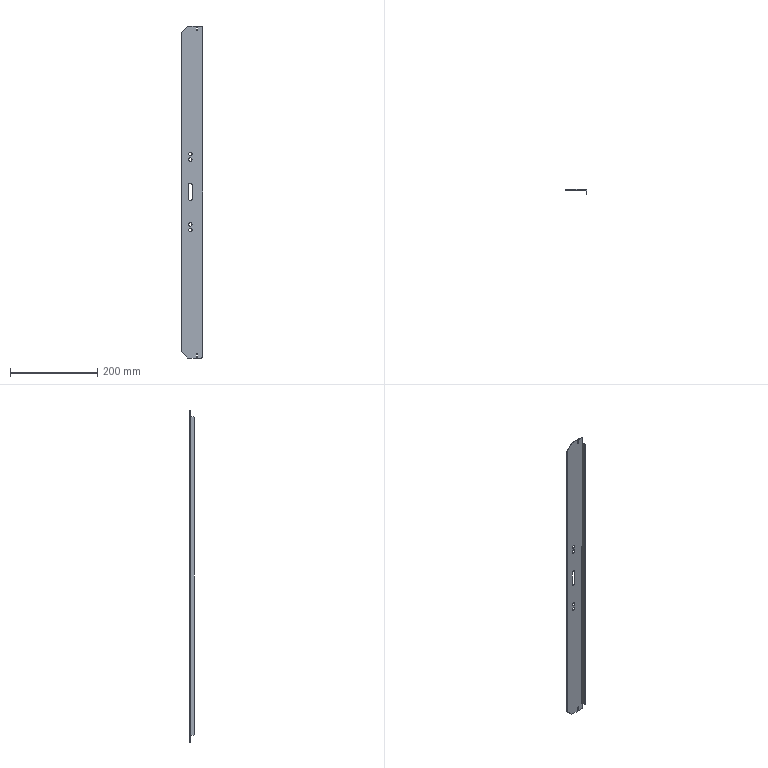Part | SolidWorks | features BaseBody 1 | 1 solid | 39 faces | box 49.5 x 10.7 x 760 mm | volume 52509 mm3 | cylinder 21 | plane 18 | commonest cylinder face diameters 8 x11 4 x6 6 x4
STEP:
#1=CARTESIAN_POINT('',(11.25,0.,378.));
#2=VERTEX_POINT('',#1);
#3=CARTESIAN_POINT('',(11.25,1.2,378.));
#4=VERTEX_POINT('',#3);
#5=CARTESIAN_POINT('',(11.25,-9.501,378.));
#6=DIRECTION('',(0.,1.,0.));
#7=VECTOR('',#6,1000.);
#8=LINE('',#5,#7);
#9=EDGE_CURVE('',#2,#4,#8,.T.);
#10=ORIENTED_EDGE('',*,*,#9,.F.);
#11=CARTESIAN_POINT('',(9.25,0.,376.));
#12=VERTEX_POINT('',#11);
#13=CARTESIAN_POINT('',(11.25,0.,376.));
#14=DIRECTION('',(0.,-1.,0.));
#15=DIRECTION('',(0.,0.,1.));
#16=AXIS2_PLACEMENT_3D('',#13,#14,#15);
#17=CIRCLE('',#16,2.);
#18=EDGE_CURVE('',#2,#12,#17,.T.);
#19=ORIENTED_EDGE('',*,*,#18,.T.);
#20=CARTESIAN_POINT('',(9.25,1.2,376.));
#21=VERTEX_POINT('',#20);
#22=CARTESIAN_POINT('',(9.25,-9.501,376.));
#23=DIRECTION('',(0.,1.,0.));
#24=VECTOR('',#23,1000.);
#25=LINE('',#22,#24);
#26=EDGE_CURVE('',#12,#21,#25,.T.);
#27=ORIENTED_EDGE('',*,*,#26,.T.);
#28=CARTESIAN_POINT('',(11.25,1.2,376.));
#29=DIRECTION('',(0.,1.,0.));
#30=DIRECTION('',(0.,0.,1.));
#31=AXIS2_PLACEMENT_3D('',#28,#29,#30);
#32=CIRCLE('',#31,2.);
#33=EDGE_CURVE('',#21,#4,#32,.T.);
#34=ORIENTED_EDGE('',*,*,#33,.T.);
#35=EDGE_LOOP('',(#10,#19,#27,#34));
#36=FACE_OUTER_BOUND('',#35,.T.);
#37=CARTESIAN_POINT('',(11.25,-9.501,376.));
#38=DIRECTION('',(0.,1.,0.));
#39=DIRECTION('',(0.,0.,1.));
#40=AXIS2_PLACEMENT_3D('',#37,#38,#39);
#41=CYLINDRICAL_SURFACE('',#40,2.);
#42=ADVANCED_FACE('',(#36),#41,.F.);
#43=CARTESIAN_POINT('',(9.25,0.,-376.));
#44=VERTEX_POINT('',#43);
#45=CARTESIAN_POINT('',(13.25,0.,-376.));
#46=VERTEX_POINT('',#45);
#47=CARTESIAN_POINT('',(11.25,0.,-376.));
#48=DIRECTION('',(0.,-1.,0.));
#49=DIRECTION('',(0.,0.,1.));
#50=AXIS2_PLACEMENT_3D('',#47,#48,#49);
#51=CIRCLE('',#50,2.);
#52=EDGE_CURVE('',#44,#46,#51,.T.);
#53=ORIENTED_EDGE('',*,*,#52,.T.);
#54=CARTESIAN_POINT('',(13.25,1.2,-376.));
#55=VERTEX_POINT('',#54);
#56=CARTESIAN_POINT('',(13.25,-9.501,-376.));
#57=DIRECTION('',(0.,1.,0.));
#58=VECTOR('',#57,1000.);
#59=LINE('',#56,#58);
#60=EDGE_CURVE('',#46,#55,#59,.T.);
#61=ORIENTED_EDGE('',*,*,#60,.T.);
#62=CARTESIAN_POINT('',(9.25,1.2,-376.));
#63=VERTEX_POINT('',#62);
#64=CARTESIAN_POINT('',(11.25,1.2,-376.));
#65=DIRECTION('',(0.,1.,0.));
#66=DIRECTION('',(0.,0.,1.));
#67=AXIS2_PLACEMENT_3D('',#64,#65,#66);
#68=CIRCLE('',#67,2.);
#69=EDGE_CURVE('',#55,#63,#68,.T.);
#70=ORIENTED_EDGE('',*,*,#69,.T.);
#71=CARTESIAN_POINT('',(9.25,-9.501,-376.));
#72=DIRECTION('',(0.,1.,0.));
#73=VECTOR('',#72,1000.);
#74=LINE('',#71,#73);
#75=EDGE_CURVE('',#44,#63,#74,.T.);
#76=ORIENTED_EDGE('',*,*,#75,.F.);
#77=EDGE_LOOP('',(#53,#61,#70,#76));
#78=FACE_OUTER_BOUND('',#77,.T.);
#79=CARTESIAN_POINT('',(11.25,-9.501,-376.));
#80=DIRECTION('',(0.,1.,0.));
#81=DIRECTION('',(0.,0.,1.));
#82=AXIS2_PLACEMENT_3D('',#79,#80,#81);
#83=CYLINDRICAL_SURFACE('',#82,2.);
#84=ADVANCED_FACE('',(#78),#83,.F.);
#85=CARTESIAN_POINT('',(13.25,0.,-372.));
#86=VERTEX_POINT('',#85);
#87=CARTESIAN_POINT('',(13.25,0.,-376.));
#88=DIRECTION('',(0.,0.,1.));
#89=VECTOR('',#88,1000.);
#90=LINE('',#87,#89);
#91=EDGE_CURVE('',#46,#86,#90,.T.);
#92=ORIENTED_EDGE('',*,*,#91,.T.);
#93=CARTESIAN_POINT('',(13.25,1.2,-372.));
#94=VERTEX_POINT('',#93);
#95=CARTESIAN_POINT('',(13.25,-9.501,-372.));
#96=DIRECTION('',(0.,1.,0.));
#97=VECTOR('',#96,1000.);
#98=LINE('',#95,#97);
#99=EDGE_CURVE('',#86,#94,#98,.T.);
#100=ORIENTED_EDGE('',*,*,#99,.T.);
#101=CARTESIAN_POINT('',(13.25,1.2,-376.));
#102=DIRECTION('',(0.,0.,-1.));
#103=VECTOR('',#102,1000.);
#104=LINE('',#101,#103);
#105=EDGE_CURVE('',#94,#55,#104,.T.);
#106=ORIENTED_EDGE('',*,*,#105,.T.);
#107=ORIENTED_EDGE('',*,*,#60,.F.);
#108=EDGE_LOOP('',(#92,#100,#106,#107));
#109=FACE_OUTER_BOUND('',#108,.T.);
#110=CARTESIAN_POINT('',(13.25,-9.501,-376.));
#111=DIRECTION('',(1.,0.,0.));
#112=DIRECTION('',(0.,0.,-1.));
#113=AXIS2_PLACEMENT_3D('',#110,#111,#112);
#114=PLANE('',#113);
#115=ADVANCED_FACE('',(#109),#114,.F.);
#116=CARTESIAN_POINT('',(11.25,0.,-370.));
#117=VERTEX_POINT('',#116);
#118=CARTESIAN_POINT('',(11.25,1.2,-370.));
#119=VERTEX_POINT('',#118);
#120=CARTESIAN_POINT('',(11.25,-9.501,-370.));
#121=DIRECTION('',(0.,1.,0.));
#122=VECTOR('',#121,1000.);
#123=LINE('',#120,#122);
#124=EDGE_CURVE('',#117,#119,#123,.T.);
#125=ORIENTED_EDGE('',*,*,#124,.F.);
#126=CARTESIAN_POINT('',(9.25,0.,-372.));
#127=VERTEX_POINT('',#126);
#128=CARTESIAN_POINT('',(11.25,0.,-372.));
#129=DIRECTION('',(0.,-1.,0.));
#130=DIRECTION('',(0.,0.,1.));
#131=AXIS2_PLACEMENT_3D('',#128,#129,#130);
#132=CIRCLE('',#131,2.);
#133=EDGE_CURVE('',#117,#127,#132,.T.);
#134=ORIENTED_EDGE('',*,*,#133,.T.);
#135=CARTESIAN_POINT('',(9.25,1.2,-372.));
#136=VERTEX_POINT('',#135);
#137=CARTESIAN_POINT('',(9.25,-9.501,-372.));
#138=DIRECTION('',(0.,1.,0.));
#139=VECTOR('',#138,1000.);
#140=LINE('',#137,#139);
#141=EDGE_CURVE('',#127,#136,#140,.T.);
#142=ORIENTED_EDGE('',*,*,#141,.T.);
#143=CARTESIAN_POINT('',(11.25,1.2,-372.));
#144=DIRECTION('',(0.,1.,0.));
#145=DIRECTION('',(0.,0.,1.));
#146=AXIS2_PLACEMENT_3D('',#143,#144,#145);
#147=CIRCLE('',#146,2.);
#148=EDGE_CURVE('',#136,#119,#147,.T.);
#149=ORIENTED_EDGE('',*,*,#148,.T.);
#150=EDGE_LOOP('',(#125,#134,#142,#149));
#151=FACE_OUTER_BOUND('',#150,.T.);
#152=CARTESIAN_POINT('',(11.25,-9.501,-372.));
#153=DIRECTION('',(0.,1.,0.));
#154=DIRECTION('',(0.,0.,1.));
#155=AXIS2_PLACEMENT_3D('',#152,#153,#154);
#156=CYLINDRICAL_SURFACE('',#155,2.);
#157=ADVANCED_FACE('',(#151),#156,.F.);
#158=CARTESIAN_POINT('',(9.25,0.,-376.));
#159=DIRECTION('',(0.,0.,-1.));
#160=VECTOR('',#159,1000.);
#161=LINE('',#158,#160);
#162=EDGE_CURVE('',#127,#44,#161,.T.);
#163=ORIENTED_EDGE('',*,*,#162,.T.);
#164=ORIENTED_EDGE('',*,*,#75,.T.);
#165=CARTESIAN_POINT('',(9.25,1.2,-376.));
#166=DIRECTION('',(0.,0.,1.));
#167=VECTOR('',#166,1000.);
#168=LINE('',#165,#167);
#169=EDGE_CURVE('',#63,#136,#168,.T.);
#170=ORIENTED_EDGE('',*,*,#169,.T.);
#171=ORIENTED_EDGE('',*,*,#141,.F.);
#172=EDGE_LOOP('',(#163,#164,#170,#171));
#173=FACE_OUTER_BOUND('',#172,.T.);
#174=CARTESIAN_POINT('',(9.25,-9.501,-376.));
#175=DIRECTION('',(-1.,0.,0.));
#176=DIRECTION('',(0.,1.,0.));
#177=AXIS2_PLACEMENT_3D('',#174,#175,#176);
#178=PLANE('',#177);
#179=ADVANCED_FACE('',(#173),#178,.F.);
#180=CARTESIAN_POINT('',(9.25,0.,372.));
#181=VERTEX_POINT('',#180);
#182=CARTESIAN_POINT('',(9.25,0.,372.));
#183=DIRECTION('',(0.,0.,-1.));
#184=VECTOR('',#183,1000.);
#185=LINE('',#182,#184);
#186=EDGE_CURVE('',#12,#181,#185,.T.);
#187=ORIENTED_EDGE('',*,*,#186,.T.);
#188=CARTESIAN_POINT('',(9.25,1.2,372.));
#189=VERTEX_POINT('',#188);
#190=CARTESIAN_POINT('',(9.25,-9.501,372.));
#191=DIRECTION('',(0.,1.,0.));
#192=VECTOR('',#191,1000.);
#193=LINE('',#190,#192);
#194=EDGE_CURVE('',#181,#189,#193,.T.);
#195=ORIENTED_EDGE('',*,*,#194,.T.);
#196=CARTESIAN_POINT('',(9.25,1.2,372.));
#197=DIRECTION('',(0.,0.,1.));
#198=VECTOR('',#197,1000.);
#199=LINE('',#196,#198);
#200=EDGE_CURVE('',#189,#21,#199,.T.);
#201=ORIENTED_EDGE('',*,*,#200,.T.);
#202=ORIENTED_EDGE('',*,*,#26,.F.);
#203=EDGE_LOOP('',(#187,#195,#201,#202));
#204=FACE_OUTER_BOUND('',#203,.T.);
#205=CARTESIAN_POINT('',(9.25,-9.501,372.));
#206=DIRECTION('',(-1.,0.,0.));
#207=DIRECTION('',(0.,1.,0.));
#208=AXIS2_PLACEMENT_3D('',#205,#206,#207);
#209=PLANE('',#208);
#210=ADVANCED_FACE('',(#204),#209,.F.);
#211=CARTESIAN_POINT('',(13.25,0.,372.));
#212=VERTEX_POINT('',#211);
#213=CARTESIAN_POINT('',(13.25,0.,376.));
#214=VERTEX_POINT('',#213);
#215=CARTESIAN_POINT('',(13.25,0.,372.));
#216=DIRECTION('',(0.,0.,1.));
#217=VECTOR('',#216,1000.);
#218=LINE('',#215,#217);
#219=EDGE_CURVE('',#212,#214,#218,.T.);
#220=ORIENTED_EDGE('',*,*,#219,.T.);
#221=CARTESIAN_POINT('',(13.25,1.2,376.));
#222=VERTEX_POINT('',#221);
#223=CARTESIAN_POINT('',(13.25,-9.501,376.));
#224=DIRECTION('',(0.,1.,0.));
#225=VECTOR('',#224,1000.);
#226=LINE('',#223,#225);
#227=EDGE_CURVE('',#214,#222,#226,.T.);
#228=ORIENTED_EDGE('',*,*,#227,.T.);
#229=CARTESIAN_POINT('',(13.25,1.2,372.));
#230=VERTEX_POINT('',#229);
#231=CARTESIAN_POINT('',(13.25,1.2,372.));
#232=DIRECTION('',(0.,0.,-1.));
#233=VECTOR('',#232,1000.);
#234=LINE('',#231,#233);
#235=EDGE_CURVE('',#222,#230,#234,.T.);
#236=ORIENTED_EDGE('',*,*,#235,.T.);
#237=CARTESIAN_POINT('',(13.25,-9.501,372.));
#238=DIRECTION('',(0.,1.,0.));
#239=VECTOR('',#238,1000.);
#240=LINE('',#237,#239);
#241=EDGE_CURVE('',#212,#230,#240,.T.);
#242=ORIENTED_EDGE('',*,*,#241,.F.);
#243=EDGE_LOOP('',(#220,#228,#236,#242));
#244=FACE_OUTER_BOUND('',#243,.T.);
#245=CARTESIAN_POINT('',(13.25,-9.501,372.));
#246=DIRECTION('',(1.,0.,0.));
#247=DIRECTION('',(0.,0.,-1.));
#248=AXIS2_PLACEMENT_3D('',#245,#246,#247);
#249=PLANE('',#248);
#250=ADVANCED_FACE('',(#244),#249,.F.);
#251=CARTESIAN_POINT('',(11.25,0.,372.));
#252=DIRECTION('',(0.,-1.,0.));
#253=DIRECTION('',(0.,0.,1.));
#254=AXIS2_PLACEMENT_3D('',#251,#252,#253);
#255=CIRCLE('',#254,2.);
#256=EDGE_CURVE('',#181,#212,#255,.T.);
#257=ORIENTED_EDGE('',*,*,#256,.T.);
#258=ORIENTED_EDGE('',*,*,#241,.T.);
#259=CARTESIAN_POINT('',(11.25,1.2,372.));
#260=DIRECTION('',(0.,1.,0.));
#261=DIRECTION('',(0.,0.,1.));
#262=AXIS2_PLACEMENT_3D('',#259,#260,#261);
#263=CIRCLE('',#262,2.);
#264=EDGE_CURVE('',#230,#189,#263,.T.);
#265=ORIENTED_EDGE('',*,*,#264,.T.);
#266=ORIENTED_EDGE('',*,*,#194,.F.);
#267=EDGE_LOOP('',(#257,#258,#265,#266));
#268=FACE_OUTER_BOUND('',#267,.T.);
#269=CARTESIAN_POINT('',(11.25,-9.501,372.));
#270=DIRECTION('',(0.,1.,0.));
#271=DIRECTION('',(0.,0.,1.));
#272=AXIS2_PLACEMENT_3D('',#269,#270,#271);
#273=CYLINDRICAL_SURFACE('',#272,2.);
#274=ADVANCED_FACE('',(#268),#273,.F.);
#275=CARTESIAN_POINT('',(-3.75,0.,83.));
#276=VERTEX_POINT('',#275);
#277=CARTESIAN_POINT('',(-3.75,1.2,83.));
#278=VERTEX_POINT('',#277);
#279=CARTESIAN_POINT('',(-3.75,-9.501,83.));
#280=DIRECTION('',(0.,1.,0.));
#281=VECTOR('',#280,1000.);
#282=LINE('',#279,#281);
#283=EDGE_CURVE('',#276,#278,#282,.T.);
#284=ORIENTED_EDGE('',*,*,#283,.F.);
#285=CARTESIAN_POINT('',(-3.75,0.,91.));
#286=VERTEX_POINT('',#285);
#287=CARTESIAN_POINT('',(-3.75,0.,87.));
#288=DIRECTION('',(0.,-1.,0.));
#289=DIRECTION('',(0.,0.,1.));
#290=AXIS2_PLACEMENT_3D('',#287,#288,#289);
#291=CIRCLE('',#290,4.);
#292=EDGE_CURVE('',#276,#286,#291,.T.);
#293=ORIENTED_EDGE('',*,*,#292,.T.);
#294=CARTESIAN_POINT('',(-3.75,1.2,91.));
#295=VERTEX_POINT('',#294);
#296=CARTESIAN_POINT('',(-3.75,-9.501,91.));
#297=DIRECTION('',(0.,1.,0.));
#298=VECTOR('',#297,1000.);
#299=LINE('',#296,#298);
#300=EDGE_CURVE('',#286,#295,#299,.T.);
#301=ORIENTED_EDGE('',*,*,#300,.T.);
#302=CARTESIAN_POINT('',(-3.75,1.2,87.));
#303=DIRECTION('',(0.,1.,0.));
#304=DIRECTION('',(0.,0.,1.));
#305=AXIS2_PLACEMENT_3D('',#302,#303,#304);
#306=CIRCLE('',#305,4.);
#307=EDGE_CURVE('',#295,#278,#306,.T.);
#308=ORIENTED_EDGE('',*,*,#307,.T.);
#309=EDGE_LOOP('',(#284,#293,#301,#308));
#310=FACE_OUTER_BOUND('',#309,.T.);
#311=CARTESIAN_POINT('',(-3.75,-9.501,87.));
#312=DIRECTION('',(0.,1.,0.));
#313=DIRECTION('',(0.,0.,1.));
#314=AXIS2_PLACEMENT_3D('',#311,#312,#313);
#315=CYLINDRICAL_SURFACE('',#314,4.);
#316=ADVANCED_FACE('',(#310),#315,.F.);
#317=CARTESIAN_POINT('',(0.25,0.,-16.));
#318=VERTEX_POINT('',#317);
#319=CARTESIAN_POINT('',(0.25,0.,16.));
#320=VERTEX_POINT('',#319);
#321=CARTESIAN_POINT('',(0.25,0.,16.));
#322=DIRECTION('',(0.,0.,1.));
#323=VECTOR('',#322,1000.);
#324=LINE('',#321,#323);
#325=EDGE_CURVE('',#318,#320,#324,.T.);
#326=ORIENTED_EDGE('',*,*,#325,.T.);
#327=CARTESIAN_POINT('',(0.25,1.2,16.));
#328=VERTEX_POINT('',#327);
#329=CARTESIAN_POINT('',(0.25,-9.501,16.));
#330=DIRECTION('',(0.,1.,0.));
#331=VECTOR('',#330,1000.);
#332=LINE('',#329,#331);
#333=EDGE_CURVE('',#320,#328,#332,.T.);
#334=ORIENTED_EDGE('',*,*,#333,.T.);
#335=CARTESIAN_POINT('',(0.25,1.2,-16.));
#336=VERTEX_POINT('',#335);
#337=CARTESIAN_POINT('',(0.25,1.2,16.));
#338=DIRECTION('',(0.,0.,-1.));
#339=VECTOR('',#338,1000.);
#340=LINE('',#337,#339);
#341=EDGE_CURVE('',#328,#336,#340,.T.);
#342=ORIENTED_EDGE('',*,*,#341,.T.);
#343=CARTESIAN_POINT('',(0.25,-9.501,-16.));
#344=DIRECTION('',(0.,1.,0.));
#345=VECTOR('',#344,1000.);
#346=LINE('',#343,#345);
#347=EDGE_CURVE('',#318,#336,#346,.T.);
#348=ORIENTED_EDGE('',*,*,#347,.F.);
#349=EDGE_LOOP('',(#326,#334,#342,#348));
#350=FACE_OUTER_BOUND('',#349,.T.);
#351=CARTESIAN_POINT('',(0.25,-9.501,16.));
#352=DIRECTION('',(1.,0.,0.));
#353=DIRECTION('',(0.,1.,0.));
#354=AXIS2_PLACEMENT_3D('',#351,#352,#353);
#355=PLANE('',#354);
#356=ADVANCED_FACE('',(#350),#355,.F.);
#357=CARTESIAN_POINT('',(-7.75,0.,-16.));
#358=VERTEX_POINT('',#357);
#359=CARTESIAN_POINT('',(-3.75,0.,-16.));
#360=DIRECTION('',(0.,-1.,0.));
#361=DIRECTION('',(0.,0.,1.));
#362=AXIS2_PLACEMENT_3D('',#359,#360,#361);
#363=CIRCLE('',#362,4.);
#364=EDGE_CURVE('',#358,#318,#363,.T.);
#365=ORIENTED_EDGE('',*,*,#364,.T.);
#366=ORIENTED_EDGE('',*,*,#347,.T.);
#367=CARTESIAN_POINT('',(-7.75,1.2,-16.));
#368=VERTEX_POINT('',#367);
#369=CARTESIAN_POINT('',(-3.75,1.2,-16.));
#370=DIRECTION('',(0.,1.,0.));
#371=DIRECTION('',(0.,0.,1.));
#372=AXIS2_PLACEMENT_3D('',#369,#370,#371);
#373=CIRCLE('',#372,4.);
#374=EDGE_CURVE('',#336,#368,#373,.T.);
#375=ORIENTED_EDGE('',*,*,#374,.T.);
#376=CARTESIAN_POINT('',(-7.75,-9.501,-16.));
#377=DIRECTION('',(0.,1.,0.));
#378=VECTOR('',#377,1000.);
#379=LINE('',#376,#378);
#380=EDGE_CURVE('',#358,#368,#379,.T.);
#381=ORIENTED_EDGE('',*,*,#380,.F.);
#382=EDGE_LOOP('',(#365,#366,#375,#381));
#383=FACE_OUTER_BOUND('',#382,.T.);
#384=CARTESIAN_POINT('',(-3.75,-9.501,-16.));
#385=DIRECTION('',(0.,1.,0.));
#386=DIRECTION('',(0.,0.,1.));
#387=AXIS2_PLACEMENT_3D('',#384,#385,#386);
#388=CYLINDRICAL_SURFACE('',#387,4.);
#389=ADVANCED_FACE('',(#383),#388,.F.);
#390=CARTESIAN_POINT('',(-7.75,0.,16.));
#391=VERTEX_POINT('',#390);
#392=CARTESIAN_POINT('',(-7.75,0.,16.));
#393=DIRECTION('',(0.,0.,-1.));
#394=VECTOR('',#393,1000.);
#395=LINE('',#392,#394);
#396=EDGE_CURVE('',#391,#358,#395,.T.);
#397=ORIENTED_EDGE('',*,*,#396,.T.);
#398=ORIENTED_EDGE('',*,*,#380,.T.);
#399=CARTESIAN_POINT('',(-7.75,1.2,16.));
#400=VERTEX_POINT('',#399);
#401=CARTESIAN_POINT('',(-7.75,1.2,16.));
#402=DIRECTION('',(0.,0.,1.));
#403=VECTOR('',#402,1000.);
#404=LINE('',#401,#403);
#405=EDGE_CURVE('',#368,#400,#404,.T.);
#406=ORIENTED_EDGE('',*,*,#405,.T.);
#407=CARTESIAN_POINT('',(-7.75,-9.501,16.));
#408=DIRECTION('',(0.,1.,0.));
#409=VECTOR('',#408,1000.);
#410=LINE('',#407,#409);
#411=EDGE_CURVE('',#391,#400,#410,.T.);
#412=ORIENTED_EDGE('',*,*,#411,.F.);
#413=EDGE_LOOP('',(#397,#398,#406,#412));
#414=FACE_OUTER_BOUND('',#413,.T.);
#415=CARTESIAN_POINT('',(-7.75,-9.501,16.));
#416=DIRECTION('',(-1.,0.,0.));
#417=DIRECTION('',(0.,0.,1.));
#418=AXIS2_PLACEMENT_3D('',#415,#416,#417);
#419=PLANE('',#418);
#420=ADVANCED_FACE('',(#414),#419,.F.);
#421=CARTESIAN_POINT('',(-3.75,0.,20.));
#422=VERTEX_POINT('',#421);
#423=CARTESIAN_POINT('',(-3.75,1.2,20.));
#424=VERTEX_POINT('',#423);
#425=CARTESIAN_POINT('',(-3.75,-9.501,20.));
#426=DIRECTION('',(0.,1.,0.));
#427=VECTOR('',#426,1000.);
#428=LINE('',#425,#427);
#429=EDGE_CURVE('',#422,#424,#428,.T.);
#430=ORIENTED_EDGE('',*,*,#429,.F.);
#431=CARTESIAN_POINT('',(-3.75,0.,16.));
#432=DIRECTION('',(0.,-1.,0.));
#433=DIRECTION('',(0.,0.,1.));
#434=AXIS2_PLACEMENT_3D('',#431,#432,#433);
#435=CIRCLE('',#434,4.);
#436=EDGE_CURVE('',#422,#391,#435,.T.);
#437=ORIENTED_EDGE('',*,*,#436,.T.);
#438=ORIENTED_EDGE('',*,*,#411,.T.);
#439=CARTESIAN_POINT('',(-3.75,1.2,16.));
#440=DIRECTION('',(0.,1.,0.));
#441=DIRECTION('',(0.,0.,1.));
#442=AXIS2_PLACEMENT_3D('',#439,#440,#441);
#443=CIRCLE('',#442,4.);
#444=EDGE_CURVE('',#400,#424,#443,.T.);
#445=ORIENTED_EDGE('',*,*,#444,.T.);
#446=EDGE_LOOP('',(#430,#437,#438,#445));
#447=FACE_OUTER_BOUND('',#446,.T.);
#448=CARTESIAN_POINT('',(-3.75,-9.501,16.));
#449=DIRECTION('',(0.,1.,0.));
#450=DIRECTION('',(0.,0.,1.));
#451=AXIS2_PLACEMENT_3D('',#448,#449,#450);
#452=CYLINDRICAL_SURFACE('',#451,4.);
#453=ADVANCED_FACE('',(#447),#452,.F.);
#454=CARTESIAN_POINT('',(-3.75,0.,-78.));
#455=VERTEX_POINT('',#454);
#456=CARTESIAN_POINT('',(-3.75,1.2,-78.));
#457=VERTEX_POINT('',#456);
#458=CARTESIAN_POINT('',(-3.75,-9.501,-78.));
#459=DIRECTION('',(0.,1.,0.));
#460=VECTOR('',#459,1000.);
#461=LINE('',#458,#460);
#462=EDGE_CURVE('',#455,#457,#461,.T.);
#463=ORIENTED_EDGE('',*,*,#462,.F.);
#464=CARTESIAN_POINT('',(-3.75,0.,-70.));
#465=VERTEX_POINT('',#464);
#466=CARTESIAN_POINT('',(-3.75,0.,-74.));
#467=DIRECTION('',(0.,-1.,0.));
#468=DIRECTION('',(0.,0.,1.));
#469=AXIS2_PLACEMENT_3D('',#466,#467,#468);
#470=CIRCLE('',#469,4.);
#471=EDGE_CURVE('',#455,#465,#470,.T.);
#472=ORIENTED_EDGE('',*,*,#471,.T.);
#473=CARTESIAN_POINT('',(-3.75,1.2,-70.));
#474=VERTEX_POINT('',#473);
#475=CARTESIAN_POINT('',(-3.75,-9.501,-70.));
#476=DIRECTION('',(0.,1.,0.));
#477=VECTOR('',#476,1000.);
#478=LINE('',#475,#477);
#479=EDGE_CURVE('',#465,#474,#478,.T.);
#480=ORIENTED_EDGE('',*,*,#479,.T.);
#481=CARTESIAN_POINT('',(-3.75,1.2,-74.));
#482=DIRECTION('',(0.,1.,0.));
#483=DIRECTION('',(0.,0.,-1.));
#484=AXIS2_PLACEMENT_3D('',#481,#482,#483);
#485=CIRCLE('',#484,4.);
#486=EDGE_CURVE('',#474,#457,#485,.T.);
#487=ORIENTED_EDGE('',*,*,#486,.T.);
#488=EDGE_LOOP('',(#463,#472,#480,#487));
#489=FACE_OUTER_BOUND('',#488,.T.);
#490=CARTESIAN_POINT('',(-3.75,-9.501,-74.));
#491=DIRECTION('',(0.,1.,0.));
#492=DIRECTION('',(0.,0.,1.));
#493=AXIS2_PLACEMENT_3D('',#490,#491,#492);
#494=CYLINDRICAL_SURFACE('',#493,4.);
#495=ADVANCED_FACE('',(#489),#494,.F.);
#496=CARTESIAN_POINT('',(-3.75,0.,-91.));
#497=VERTEX_POINT('',#496);
#498=CARTESIAN_POINT('',(-3.75,1.2,-91.));
#499=VERTEX_POINT('',#498);
#500=CARTESIAN_POINT('',(-3.75,-9.501,-91.));
#501=DIRECTION('',(0.,1.,0.));
#502=VECTOR('',#501,1000.);
#503=LINE('',#500,#502);
#504=EDGE_CURVE('',#497,#499,#503,.T.);
#505=ORIENTED_EDGE('',*,*,#504,.F.);
#506=CARTESIAN_POINT('',(-3.75,0.,-83.));
#507=VERTEX_POINT('',#506);
#508=CARTESIAN_POINT('',(-3.75,0.,-87.));
#509=DIRECTION('',(0.,-1.,0.));
#510=DIRECTION('',(0.,0.,1.));
#511=AXIS2_PLACEMENT_3D('',#508,#509,#510);
#512=CIRCLE('',#511,4.);
#513=EDGE_CURVE('',#497,#507,#512,.T.);
#514=ORIENTED_EDGE('',*,*,#513,.T.);
#515=CARTESIAN_POINT('',(-3.75,1.2,-83.));
#516=VERTEX_POINT('',#515);
#517=CARTESIAN_POINT('',(-3.75,-9.501,-83.));
#518=DIRECTION('',(0.,1.,0.));
#519=VECTOR('',#518,1000.);
#520=LINE('',#517,#519);
#521=EDGE_CURVE('',#507,#516,#520,.T.);
#522=ORIENTED_EDGE('',*,*,#521,.T.);
#523=CARTESIAN_POINT('',(-3.75,1.2,-87.));
#524=DIRECTION('',(0.,1.,0.));
#525=DIRECTION('',(0.,0.,-1.));
#526=AXIS2_PLACEMENT_3D('',#523,#524,#525);
#527=CIRCLE('',#526,4.);
#528=EDGE_CURVE('',#516,#499,#527,.T.);
#529=ORIENTED_EDGE('',*,*,#528,.T.);
#530=EDGE_LOOP('',(#505,#514,#522,#529));
#531=FACE_OUTER_BOUND('',#530,.T.);
#532=CARTESIAN_POINT('',(-3.75,-9.501,-87.));
#533=DIRECTION('',(0.,1.,0.));
#534=DIRECTION('',(0.,0.,1.));
#535=AXIS2_PLACEMENT_3D('',#532,#533,#534);
#536=CYLINDRICAL_SURFACE('',#535,4.);
#537=ADVANCED_FACE('',(#531),#536,.F.);
#538=CARTESIAN_POINT('',(-3.75,0.,70.));
#539=VERTEX_POINT('',#538);
#540=CARTESIAN_POINT('',(-3.75,1.2,70.));
#541=VERTEX_POINT('',#540);
#542=CARTESIAN_POINT('',(-3.75,-9.501,70.));
#543=DIRECTION('',(0.,1.,0.));
#544=VECTOR('',#543,1000.);
#545=LINE('',#542,#544);
#546=EDGE_CURVE('',#539,#541,#545,.T.);
#547=ORIENTED_EDGE('',*,*,#546,.F.);
#548=CARTESIAN_POINT('',(-3.75,0.,78.));
#549=VERTEX_POINT('',#548);
#550=CARTESIAN_POINT('',(-3.75,0.,74.));
#551=DIRECTION('',(0.,-1.,0.));
#552=DIRECTION('',(0.,0.,1.));
#553=AXIS2_PLACEMENT_3D('',#550,#551,#552);
#554=CIRCLE('',#553,4.);
#555=EDGE_CURVE('',#539,#549,#554,.T.);
#556=ORIENTED_EDGE('',*,*,#555,.T.);
#557=CARTESIAN_POINT('',(-3.75,1.2,78.));
#558=VERTEX_POINT('',#557);
#559=CARTESIAN_POINT('',(-3.75,-9.501,78.));
#560=DIRECTION('',(0.,1.,0.));
#561=VECTOR('',#560,1000.);
#562=LINE('',#559,#561);
#563=EDGE_CURVE('',#549,#558,#562,.T.);
#564=ORIENTED_EDGE('',*,*,#563,.T.);
#565=CARTESIAN_POINT('',(-3.75,1.2,74.));
#566=DIRECTION('',(0.,1.,0.));
#567=DIRECTION('',(0.,0.,1.));
#568=AXIS2_PLACEMENT_3D('',#565,#566,#567);
#569=CIRCLE('',#568,4.);
#570=EDGE_CURVE('',#558,#541,#569,.T.);
#571=ORIENTED_EDGE('',*,*,#570,.T.);
#572=EDGE_LOOP('',(#547,#556,#564,#571));
#573=FACE_OUTER_BOUND('',#572,.T.);
#574=CARTESIAN_POINT('',(-3.75,-9.501,74.));
#575=DIRECTION('',(0.,1.,0.));
#576=DIRECTION('',(0.,0.,1.));
#577=AXIS2_PLACEMENT_3D('',#574,#575,#576);
#578=CYLINDRICAL_SURFACE('',#577,4.);
#579=ADVANCED_FACE('',(#573),#578,.F.);
#580=CARTESIAN_POINT('',(24.75,-6.5,365.));
#581=VERTEX_POINT('',#580);
#582=CARTESIAN_POINT('',(24.75,-9.5,362.));
#583=VERTEX_POINT('',#582);
#584=CARTESIAN_POINT('',(24.75,-6.5,362.));
#585=DIRECTION('',(1.,0.,0.));
#586=DIRECTION('',(0.,0.,1.));
#587=AXIS2_PLACEMENT_3D('',#584,#585,#586);
#588=CIRCLE('',#587,3.);
#589=EDGE_CURVE('',#581,#583,#588,.T.);
#590=ORIENTED_EDGE('',*,*,#589,.F.);
#591=CARTESIAN_POINT('',(23.55,-6.5,365.));
#592=VERTEX_POINT('',#591);
#593=CARTESIAN_POINT('',(24.75,-6.5,365.));
#594=DIRECTION('',(1.,0.,0.));
#595=VECTOR('',#594,1000.);
#596=LINE('',#593,#595);
#597=EDGE_CURVE('',#592,#581,#596,.T.);
#598=ORIENTED_EDGE('',*,*,#597,.F.);
#599=CARTESIAN_POINT('',(23.55,-9.5,362.));
#600=VERTEX_POINT('',#599);
#601=CARTESIAN_POINT('',(23.55,-6.5,362.));
#602=DIRECTION('',(-1.,0.,0.));
#603=DIRECTION('',(0.,0.,-1.));
#604=AXIS2_PLACEMENT_3D('',#601,#602,#603);
#605=CIRCLE('',#604,3.);
#606=EDGE_CURVE('',#600,#592,#605,.T.);
#607=ORIENTED_EDGE('',*,*,#606,.F.);
#608=CARTESIAN_POINT('',(0.,-9.5,362.));
#609=DIRECTION('',(-1.,0.,0.));
#610=VECTOR('',#609,1000.);
#611=LINE('',#608,#610);
#612=EDGE_CURVE('',#583,#600,#611,.T.);
#613=ORIENTED_EDGE('',*,*,#612,.F.);
#614=EDGE_LOOP('',(#590,#598,#607,#613));
#615=FACE_OUTER_BOUND('',#614,.T.);
#616=CARTESIAN_POINT('',(0.,-6.5,362.));
#617=DIRECTION('',(-1.,0.,0.));
#618=DIRECTION('',(0.,0.,1.));
#619=AXIS2_PLACEMENT_3D('',#616,#617,#618);
#620=CYLINDRICAL_SURFACE('',#619,3.);
#621=ADVANCED_FACE('',(#615),#620,.T.);
#622=CARTESIAN_POINT('',(21.75,1.2,380.));
#623=VERTEX_POINT('',#622);
#624=CARTESIAN_POINT('',(24.75,1.2,377.));
#625=VERTEX_POINT('',#624);
#626=CARTESIAN_POINT('',(21.75,1.2,377.));
#627=DIRECTION('',(0.,1.,0.));
#628=DIRECTION('',(0.,0.,1.));
#629=AXIS2_PLACEMENT_3D('',#626,#627,#628);
#630=CIRCLE('',#629,3.);
#631=EDGE_CURVE('',#623,#625,#630,.T.);
#632=ORIENTED_EDGE('',*,*,#631,.F.);
#633=CARTESIAN_POINT('',(21.75,0.,380.));
#634=VERTEX_POINT('',#633);
#635=CARTESIAN_POINT('',(21.75,1.2,380.));
#636=DIRECTION('',(0.,1.,0.));
#637=VECTOR('',#636,1000.);
#638=LINE('',#635,#637);
#639=EDGE_CURVE('',#634,#623,#638,.T.);
#640=ORIENTED_EDGE('',*,*,#639,.F.);
#641=CARTESIAN_POINT('',(24.75,0.,377.));
#642=VERTEX_POINT('',#641);
#643=CARTESIAN_POINT('',(21.75,0.,377.));
#644=DIRECTION('',(0.,-1.,0.));
#645=DIRECTION('',(0.,0.,1.));
#646=AXIS2_PLACEMENT_3D('',#643,#644,#645);
#647=CIRCLE('',#646,3.);
#648=EDGE_CURVE('',#642,#634,#647,.T.);
#649=ORIENTED_EDGE('',*,*,#648,.F.);
#650=CARTESIAN_POINT('',(24.75,1.2,377.));
#651=DIRECTION('',(0.,-1.,0.));
#652=VECTOR('',#651,1000.);
#653=LINE('',#650,#652);
#654=EDGE_CURVE('',#625,#642,#653,.T.);
#655=ORIENTED_EDGE('',*,*,#654,.F.);
#656=EDGE_LOOP('',(#632,#640,#649,#655));
#657=FACE_OUTER_BOUND('',#656,.T.);
#658=CARTESIAN_POINT('',(21.75,1.2,377.));
#659=DIRECTION('',(0.,-1.,0.));
#660=DIRECTION('',(0.,0.,-1.));
#661=AXIS2_PLACEMENT_3D('',#658,#659,#660);
#662=CYLINDRICAL_SURFACE('',#661,3.);
#663=ADVANCED_FACE('',(#657),#662,.T.);
#664=CARTESIAN_POINT('',(24.75,-9.5,-362.));
#665=VERTEX_POINT('',#664);
#666=CARTESIAN_POINT('',(24.75,-6.5,-365.));
#667=VERTEX_POINT('',#666);
#668=CARTESIAN_POINT('',(24.75,-6.5,-362.));
#669=DIRECTION('',(1.,0.,0.));
#670=DIRECTION('',(0.,0.,1.));
#671=AXIS2_PLACEMENT_3D('',#668,#669,#670);
#672=CIRCLE('',#671,3.);
#673=EDGE_CURVE('',#665,#667,#672,.T.);
#674=ORIENTED_EDGE('',*,*,#673,.F.);
#675=CARTESIAN_POINT('',(23.55,-9.5,-362.));
#676=VERTEX_POINT('',#675);
#677=CARTESIAN_POINT('',(0.,-9.5,-362.));
#678=DIRECTION('',(1.,0.,0.));
#679=VECTOR('',#678,1000.);
#680=LINE('',#677,#679);
#681=EDGE_CURVE('',#676,#665,#680,.T.);
#682=ORIENTED_EDGE('',*,*,#681,.F.);
#683=CARTESIAN_POINT('',(23.55,-6.5,-365.));
#684=VERTEX_POINT('',#683);
#685=CARTESIAN_POINT('',(23.55,-6.5,-362.));
#686=DIRECTION('',(-1.,0.,0.));
#687=DIRECTION('',(0.,0.,-1.));
#688=AXIS2_PLACEMENT_3D('',#685,#686,#687);
#689=CIRCLE('',#688,3.);
#690=EDGE_CURVE('',#684,#676,#689,.T.);
#691=ORIENTED_EDGE('',*,*,#690,.F.);
#692=CARTESIAN_POINT('',(24.75,-6.5,-365.));
#693=DIRECTION('',(-1.,0.,0.));
#694=VECTOR('',#693,1000.);
#695=LINE('',#692,#694);
#696=EDGE_CURVE('',#667,#684,#695,.T.);
#697=ORIENTED_EDGE('',*,*,#696,.F.);
#698=EDGE_LOOP('',(#674,#682,#691,#697));
#699=FACE_OUTER_BOUND('',#698,.T.);
#700=CARTESIAN_POINT('',(24.75,-6.5,-362.));
#701=DIRECTION('',(-1.,0.,0.));
#702=DIRECTION('',(0.,0.,1.));
#703=AXIS2_PLACEMENT_3D('',#700,#701,#702);
#704=CYLINDRICAL_SURFACE('',#703,3.);
#705=ADVANCED_FACE('',(#699),#704,.T.);
#706=CARTESIAN_POINT('',(24.75,1.2,-377.));
#707=VERTEX_POINT('',#706);
#708=CARTESIAN_POINT('',(21.75,1.2,-380.));
#709=VERTEX_POINT('',#708);
#710=CARTESIAN_POINT('',(21.75,1.2,-377.));
#711=DIRECTION('',(0.,1.,0.));
#712=DIRECTION('',(0.,0.,1.));
#713=AXIS2_PLACEMENT_3D('',#710,#711,#712);
#714=CIRCLE('',#713,3.);
#715=EDGE_CURVE('',#707,#709,#714,.T.);
#716=ORIENTED_EDGE('',*,*,#715,.F.);
#717=CARTESIAN_POINT('',(24.75,0.,-377.));
#718=VERTEX_POINT('',#717);
#719=CARTESIAN_POINT('',(24.75,1.2,-377.));
#720=DIRECTION('',(0.,1.,0.));
#721=VECTOR('',#720,1000.);
#722=LINE('',#719,#721);
#723=EDGE_CURVE('',#718,#707,#722,.T.);
#724=ORIENTED_EDGE('',*,*,#723,.F.);
#725=CARTESIAN_POINT('',(21.75,0.,-380.));
#726=VERTEX_POINT('',#725);
#727=CARTESIAN_POINT('',(21.75,0.,-377.));
#728=DIRECTION('',(0.,-1.,0.));
#729=DIRECTION('',(0.,0.,1.));
#730=AXIS2_PLACEMENT_3D('',#727,#728,#729);
#731=CIRCLE('',#730,3.);
#732=EDGE_CURVE('',#726,#718,#731,.T.);
#733=ORIENTED_EDGE('',*,*,#732,.F.);
#734=CARTESIAN_POINT('',(21.75,1.2,-380.));
#735=DIRECTION('',(0.,-1.,0.));
#736=VECTOR('',#735,1000.);
#737=LINE('',#734,#736);
#738=EDGE_CURVE('',#709,#726,#737,.T.);
#739=ORIENTED_EDGE('',*,*,#738,.F.);
#740=EDGE_LOOP('',(#716,#724,#733,#739));
#741=FACE_OUTER_BOUND('',#740,.T.);
#742=CARTESIAN_POINT('',(21.75,1.2,-377.));
#743=DIRECTION('',(0.,-1.,0.));
#744=DIRECTION('',(0.,0.,-1.));
#745=AXIS2_PLACEMENT_3D('',#742,#743,#744);
#746=CYLINDRICAL_SURFACE('',#745,3.);
#747=ADVANCED_FACE('',(#741),#746,.T.);
#748=CARTESIAN_POINT('',(24.75,0.,-365.));
#749=VERTEX_POINT('',#748);
#750=CARTESIAN_POINT('',(24.75,0.,-365.));
#751=DIRECTION('',(0.,1.,0.));
#752=VECTOR('',#751,1000.);
#753=LINE('',#750,#752);
#754=EDGE_CURVE('',#667,#749,#753,.T.);
#755=ORIENTED_EDGE('',*,*,#754,.F.);
#756=ORIENTED_EDGE('',*,*,#696,.T.);
#757=CARTESIAN_POINT('',(23.55,0.,-365.));
#758=VERTEX_POINT('',#757);
#759=CARTESIAN_POINT('',(23.55,0.,-365.));
#760=DIRECTION('',(0.,1.,0.));
#761=VECTOR('',#760,1000.);
#762=LINE('',#759,#761);
#763=EDGE_CURVE('',#684,#758,#762,.T.);
#764=ORIENTED_EDGE('',*,*,#763,.T.);
#765=CARTESIAN_POINT('',(24.75,0.,-365.));
#766=DIRECTION('',(-1.,0.,0.));
#767=VECTOR('',#766,1000.);
#768=LINE('',#765,#767);
#769=EDGE_CURVE('',#749,#758,#768,.T.);
#770=ORIENTED_EDGE('',*,*,#769,.F.);
#771=EDGE_LOOP('',(#755,#756,#764,#770));
#772=FACE_OUTER_BOUND('',#771,.T.);
#773=CARTESIAN_POINT('',(24.75,0.,-365.));
#774=DIRECTION('',(0.,0.,1.));
#775=DIRECTION('',(1.,0.,0.));
#776=AXIS2_PLACEMENT_3D('',#773,#774,#775);
#777=PLANE('',#776);
#778=ADVANCED_FACE('',(#772),#777,.F.);
#779=CARTESIAN_POINT('',(23.55,0.,365.));
#780=VERTEX_POINT('',#779);
#781=CARTESIAN_POINT('',(23.55,0.,365.));
#782=DIRECTION('',(0.,-1.,0.));
#783=VECTOR('',#782,1000.);
#784=LINE('',#781,#783);
#785=EDGE_CURVE('',#780,#592,#784,.T.);
#786=ORIENTED_EDGE('',*,*,#785,.T.);
#787=ORIENTED_EDGE('',*,*,#597,.T.);
#788=CARTESIAN_POINT('',(24.75,0.,365.));
#789=VERTEX_POINT('',#788);
#790=CARTESIAN_POINT('',(24.75,0.,365.));
#791=DIRECTION('',(0.,-1.,0.));
#792=VECTOR('',#791,1000.);
#793=LINE('',#790,#792);
#794=EDGE_CURVE('',#789,#581,#793,.T.);
#795=ORIENTED_EDGE('',*,*,#794,.F.);
#796=CARTESIAN_POINT('',(24.75,0.,365.));
#797=DIRECTION('',(-1.,0.,0.));
#798=VECTOR('',#797,1000.);
#799=LINE('',#796,#798);
#800=EDGE_CURVE('',#789,#780,#799,.T.);
#801=ORIENTED_EDGE('',*,*,#800,.T.);
#802=EDGE_LOOP('',(#786,#787,#795,#801));
#803=FACE_OUTER_BOUND('',#802,.T.);
#804=CARTESIAN_POINT('',(24.75,0.,365.));
#805=DIRECTION('',(0.,0.,-1.));
#806=DIRECTION('',(-1.,0.,0.));
#807=AXIS2_PLACEMENT_3D('',#804,#805,#806);
#808=PLANE('',#807);
#809=ADVANCED_FACE('',(#803),#808,.F.);
#810=CARTESIAN_POINT('',(23.55,-9.5,380.));
#811=DIRECTION('',(0.,0.,-1.));
#812=VECTOR('',#811,1000.);
#813=LINE('',#810,#812);
#814=EDGE_CURVE('',#600,#676,#813,.T.);
#815=ORIENTED_EDGE('',*,*,#814,.T.);
#816=ORIENTED_EDGE('',*,*,#681,.T.);
#817=CARTESIAN_POINT('',(24.75,-9.5,380.));
#818=DIRECTION('',(0.,0.,-1.));
#819=VECTOR('',#818,1000.);
#820=LINE('',#817,#819);
#821=EDGE_CURVE('',#583,#665,#820,.T.);
#822=ORIENTED_EDGE('',*,*,#821,.F.);
#823=ORIENTED_EDGE('',*,*,#612,.T.);
#824=EDGE_LOOP('',(#815,#816,#822,#823));
#825=FACE_OUTER_BOUND('',#824,.T.);
#826=CARTESIAN_POINT('',(0.,-9.5,0.));
#827=DIRECTION('',(0.,1.,0.));
#828=DIRECTION('',(1.,0.,0.));
#829=AXIS2_PLACEMENT_3D('',#826,#827,#828);
#830=PLANE('',#829);
#831=ADVANCED_FACE('',(#825),#830,.F.);
#832=ORIENTED_EDGE('',*,*,#763,.F.);
#833=ORIENTED_EDGE('',*,*,#690,.T.);
#834=ORIENTED_EDGE('',*,*,#814,.F.);
#835=ORIENTED_EDGE('',*,*,#606,.T.);
#836=ORIENTED_EDGE('',*,*,#785,.F.);
#837=CARTESIAN_POINT('',(23.55,0.,380.));
#838=DIRECTION('',(0.,0.,-1.));
#839=VECTOR('',#838,1000.);
#840=LINE('',#837,#839);
#841=EDGE_CURVE('',#780,#758,#840,.T.);
#842=ORIENTED_EDGE('',*,*,#841,.T.);
#843=EDGE_LOOP('',(#832,#833,#834,#835,#836,#842));
#844=FACE_OUTER_BOUND('',#843,.T.);
#845=CARTESIAN_POINT('',(23.55,-9.5,380.));
#846=DIRECTION('',(1.,0.,0.));
#847=DIRECTION('',(0.,0.,-1.));
#848=AXIS2_PLACEMENT_3D('',#845,#846,#847);
#849=PLANE('',#848);
#850=ADVANCED_FACE('',(#844),#849,.F.);
#851=CARTESIAN_POINT('',(-24.75,1.2,365.));
#852=VERTEX_POINT('',#851);
#853=CARTESIAN_POINT('',(-9.75,1.2,380.));
#854=VERTEX_POINT('',#853);
#855=CARTESIAN_POINT('',(-194.875,1.2,194.875));
#856=DIRECTION('',(0.7071,0.,0.7071));
#857=VECTOR('',#856,1000.);
#858=LINE('',#855,#857);
#859=EDGE_CURVE('',#852,#854,#858,.T.);
#860=ORIENTED_EDGE('',*,*,#859,.F.);
#861=CARTESIAN_POINT('',(-24.75,0.,365.));
#862=VERTEX_POINT('',#861);
#863=CARTESIAN_POINT('',(-24.75,1.2,365.));
#864=DIRECTION('',(0.,1.,0.));
#865=VECTOR('',#864,1000.);
#866=LINE('',#863,#865);
#867=EDGE_CURVE('',#862,#852,#866,.T.);
#868=ORIENTED_EDGE('',*,*,#867,.F.);
#869=CARTESIAN_POINT('',(-9.75,0.,380.));
#870=VERTEX_POINT('',#869);
#871=CARTESIAN_POINT('',(-9.75,0.,380.));
#872=DIRECTION('',(-0.7071,0.,-0.7071));
#873=VECTOR('',#872,1000.);
#874=LINE('',#871,#873);
#875=EDGE_CURVE('',#870,#862,#874,.T.);
#876=ORIENTED_EDGE('',*,*,#875,.F.);
#877=CARTESIAN_POINT('',(-9.75,1.2,380.));
#878=DIRECTION('',(0.,-1.,0.));
#879=VECTOR('',#878,1000.);
#880=LINE('',#877,#879);
#881=EDGE_CURVE('',#854,#870,#880,.T.);
#882=ORIENTED_EDGE('',*,*,#881,.F.);
#883=EDGE_LOOP('',(#860,#868,#876,#882));
#884=FACE_OUTER_BOUND('',#883,.T.);
#885=CARTESIAN_POINT('',(-9.75,1.2,380.));
#886=DIRECTION('',(0.7071,0.,-0.7071));
#887=DIRECTION('',(0.,-1.,0.));
#888=AXIS2_PLACEMENT_3D('',#885,#886,#887);
#889=PLANE('',#888);
#890=ADVANCED_FACE('',(#884),#889,.F.);
#891=CARTESIAN_POINT('',(-9.75,1.2,-380.));
#892=VERTEX_POINT('',#891);
#893=CARTESIAN_POINT('',(-24.75,1.2,-365.));
#894=VERTEX_POINT('',#893);
#895=CARTESIAN_POINT('',(-194.875,1.2,-194.875));
#896=DIRECTION('',(-0.7071,0.,0.7071));
#897=VECTOR('',#896,1000.);
#898=LINE('',#895,#897);
#899=EDGE_CURVE('',#892,#894,#898,.T.);
#900=ORIENTED_EDGE('',*,*,#899,.F.);
#901=CARTESIAN_POINT('',(-9.75,0.,-380.));
#902=VERTEX_POINT('',#901);
#903=CARTESIAN_POINT('',(-9.75,1.2,-380.));
#904=DIRECTION('',(0.,1.,0.));
#905=VECTOR('',#904,1000.);
#906=LINE('',#903,#905);
#907=EDGE_CURVE('',#902,#892,#906,.T.);
#908=ORIENTED_EDGE('',*,*,#907,.F.);
#909=CARTESIAN_POINT('',(-24.75,0.,-365.));
#910=VERTEX_POINT('',#909);
#911=CARTESIAN_POINT('',(-24.75,0.,-365.));
#912=DIRECTION('',(0.7071,0.,-0.7071));
#913=VECTOR('',#912,1000.);
#914=LINE('',#911,#913);
#915=EDGE_CURVE('',#910,#902,#914,.T.);
#916=ORIENTED_EDGE('',*,*,#915,.F.);
#917=CARTESIAN_POINT('',(-24.75,1.2,-365.));
#918=DIRECTION('',(0.,-1.,0.));
#919=VECTOR('',#918,1000.);
#920=LINE('',#917,#919);
#921=EDGE_CURVE('',#894,#910,#920,.T.);
#922=ORIENTED_EDGE('',*,*,#921,.F.);
#923=EDGE_LOOP('',(#900,#908,#916,#922));
#924=FACE_OUTER_BOUND('',#923,.T.);
#925=CARTESIAN_POINT('',(-24.75,1.2,-365.));
#926=DIRECTION('',(0.7071,0.,0.7071));
#927=DIRECTION('',(0.,-1.,0.));
#928=AXIS2_PLACEMENT_3D('',#925,#926,#927);
#929=PLANE('',#928);
#930=ADVANCED_FACE('',(#924),#929,.F.);
#931=ORIENTED_EDGE('',*,*,#570,.F.);
#932=CARTESIAN_POINT('',(-3.75,1.2,74.));
#933=DIRECTION('',(0.,1.,0.));
#934=DIRECTION('',(0.,0.,1.));
#935=AXIS2_PLACEMENT_3D('',#932,#933,#934);
#936=CIRCLE('',#935,4.);
#937=EDGE_CURVE('',#541,#558,#936,.T.);
#938=ORIENTED_EDGE('',*,*,#937,.F.);
#939=EDGE_LOOP('',(#931,#938));
#940=FACE_BOUND('',#939,.T.);
#941=ORIENTED_EDGE('',*,*,#528,.F.);
#942=CARTESIAN_POINT('',(-3.75,1.2,-87.));
#943=DIRECTION('',(0.,1.,0.));
#944=DIRECTION('',(0.,0.,-1.));
#945=AXIS2_PLACEMENT_3D('',#942,#943,#944);
#946=CIRCLE('',#945,4.);
#947=EDGE_CURVE('',#499,#516,#946,.T.);
#948=ORIENTED_EDGE('',*,*,#947,.F.);
#949=EDGE_LOOP('',(#941,#948));
#950=FACE_BOUND('',#949,.T.);
#951=ORIENTED_EDGE('',*,*,#486,.F.);
#952=CARTESIAN_POINT('',(-3.75,1.2,-74.));
#953=DIRECTION('',(0.,1.,0.));
#954=DIRECTION('',(0.,0.,-1.));
#955=AXIS2_PLACEMENT_3D('',#952,#953,#954);
#956=CIRCLE('',#955,4.);
#957=EDGE_CURVE('',#457,#474,#956,.T.);
#958=ORIENTED_EDGE('',*,*,#957,.F.);
#959=EDGE_LOOP('',(#951,#958));
#960=FACE_BOUND('',#959,.T.);
#961=ORIENTED_EDGE('',*,*,#444,.F.);
#962=ORIENTED_EDGE('',*,*,#405,.F.);
#963=ORIENTED_EDGE('',*,*,#374,.F.);
#964=ORIENTED_EDGE('',*,*,#341,.F.);
#965=CARTESIAN_POINT('',(-3.75,1.2,16.));
#966=DIRECTION('',(0.,1.,0.));
#967=DIRECTION('',(0.,0.,1.));
#968=AXIS2_PLACEMENT_3D('',#965,#966,#967);
#969=CIRCLE('',#968,4.);
#970=EDGE_CURVE('',#424,#328,#969,.T.);
#971=ORIENTED_EDGE('',*,*,#970,.F.);
#972=EDGE_LOOP('',(#961,#962,#963,#964,#971));
#973=FACE_BOUND('',#972,.T.);
#974=ORIENTED_EDGE('',*,*,#307,.F.);
#975=CARTESIAN_POINT('',(-3.75,1.2,87.));
#976=DIRECTION('',(0.,1.,0.));
#977=DIRECTION('',(0.,0.,1.));
#978=AXIS2_PLACEMENT_3D('',#975,#976,#977);
#979=CIRCLE('',#978,4.);
#980=EDGE_CURVE('',#278,#295,#979,.T.);
#981=ORIENTED_EDGE('',*,*,#980,.F.);
#982=EDGE_LOOP('',(#974,#981));
#983=FACE_BOUND('',#982,.T.);
#984=ORIENTED_EDGE('',*,*,#69,.F.);
#985=ORIENTED_EDGE('',*,*,#105,.F.);
#986=CARTESIAN_POINT('',(11.25,1.2,-372.));
#987=DIRECTION('',(0.,1.,0.));
#988=DIRECTION('',(0.,0.,1.));
#989=AXIS2_PLACEMENT_3D('',#986,#987,#988);
#990=CIRCLE('',#989,2.);
#991=EDGE_CURVE('',#119,#94,#990,.T.);
#992=ORIENTED_EDGE('',*,*,#991,.F.);
#993=ORIENTED_EDGE('',*,*,#148,.F.);
#994=ORIENTED_EDGE('',*,*,#169,.F.);
#995=EDGE_LOOP('',(#984,#985,#992,#993,#994));
#996=FACE_BOUND('',#995,.T.);
#997=ORIENTED_EDGE('',*,*,#33,.F.);
#998=ORIENTED_EDGE('',*,*,#200,.F.);
#999=ORIENTED_EDGE('',*,*,#264,.F.);
#1000=ORIENTED_EDGE('',*,*,#235,.F.);
#1001=CARTESIAN_POINT('',(11.25,1.2,376.));
#1002=DIRECTION('',(0.,1.,0.));
#1003=DIRECTION('',(0.,0.,1.));
#1004=AXIS2_PLACEMENT_3D('',#1001,#1002,#1003);
#1005=CIRCLE('',#1004,2.);
#1006=EDGE_CURVE('',#4,#222,#1005,.T.);
#1007=ORIENTED_EDGE('',*,*,#1006,.F.);
#1008=EDGE_LOOP('',(#997,#998,#999,#1000,#1007));
#1009=FACE_BOUND('',#1008,.T.);
#1010=CARTESIAN_POINT('',(24.75,1.2,-380.));
#1011=DIRECTION('',(0.,0.,-1.));
#1012=VECTOR('',#1011,1000.);
#1013=LINE('',#1010,#1012);
#1014=EDGE_CURVE('',#625,#707,#1013,.T.);
#1015=ORIENTED_EDGE('',*,*,#1014,.T.);
#1016=ORIENTED_EDGE('',*,*,#715,.T.);
#1017=CARTESIAN_POINT('',(-24.75,1.2,-380.));
#1018=DIRECTION('',(-1.,0.,0.));
#1019=VECTOR('',#1018,1000.);
#1020=LINE('',#1017,#1019);
#1021=EDGE_CURVE('',#709,#892,#1020,.T.);
#1022=ORIENTED_EDGE('',*,*,#1021,.T.);
#1023=ORIENTED_EDGE('',*,*,#899,.T.);
#1024=CARTESIAN_POINT('',(-24.75,1.2,-380.));
#1025=DIRECTION('',(0.,0.,1.));
#1026=VECTOR('',#1025,1000.);
#1027=LINE('',#1024,#1026);
#1028=EDGE_CURVE('',#894,#852,#1027,.T.);
#1029=ORIENTED_EDGE('',*,*,#1028,.T.);
#1030=ORIENTED_EDGE('',*,*,#859,.T.);
#1031=CARTESIAN_POINT('',(-24.75,1.2,380.));
#1032=DIRECTION('',(1.,0.,0.));
#1033=VECTOR('',#1032,1000.);
#1034=LINE('',#1031,#1033);
#1035=EDGE_CURVE('',#854,#623,#1034,.T.);
#1036=ORIENTED_EDGE('',*,*,#1035,.T.);
#1037=ORIENTED_EDGE('',*,*,#631,.T.);
#1038=EDGE_LOOP('',(#1015,#1016,#1022,#1023,#1029,#1030,#1036,#1037));
#1039=FACE_OUTER_BOUND('',#1038,.T.);
#1040=CARTESIAN_POINT('',(0.,1.2,0.));
#1041=DIRECTION('',(0.,1.,0.));
#1042=DIRECTION('',(1.,0.,0.));
#1043=AXIS2_PLACEMENT_3D('',#1040,#1041,#1042);
#1044=PLANE('',#1043);
#1045=ADVANCED_FACE('',(#940,#950,#960,#973,#983,#996,#1009,#1039),#1044,.T.);
#1046=CARTESIAN_POINT('',(-24.75,0.,380.));
#1047=DIRECTION('',(1.,0.,0.));
#1048=VECTOR('',#1047,1000.);
#1049=LINE('',#1046,#1048);
#1050=EDGE_CURVE('',#870,#634,#1049,.T.);
#1051=ORIENTED_EDGE('',*,*,#1050,.T.);
#1052=ORIENTED_EDGE('',*,*,#639,.T.);
#1053=ORIENTED_EDGE('',*,*,#1035,.F.);
#1054=ORIENTED_EDGE('',*,*,#881,.T.);
#1055=EDGE_LOOP('',(#1051,#1052,#1053,#1054));
#1056=FACE_OUTER_BOUND('',#1055,.T.);
#1057=CARTESIAN_POINT('',(-24.75,1.2,380.));
#1058=DIRECTION('',(0.,0.,-1.));
#1059=DIRECTION('',(0.,-1.,0.));
#1060=AXIS2_PLACEMENT_3D('',#1057,#1058,#1059);
#1061=PLANE('',#1060);
#1062=ADVANCED_FACE('',(#1056),#1061,.F.);
#1063=ORIENTED_EDGE('',*,*,#1028,.F.);
#1064=ORIENTED_EDGE('',*,*,#921,.T.);
#1065=CARTESIAN_POINT('',(-24.75,0.,-380.));
#1066=DIRECTION('',(0.,0.,1.));
#1067=VECTOR('',#1066,1000.);
#1068=LINE('',#1065,#1067);
#1069=EDGE_CURVE('',#910,#862,#1068,.T.);
#1070=ORIENTED_EDGE('',*,*,#1069,.T.);
#1071=ORIENTED_EDGE('',*,*,#867,.T.);
#1072=EDGE_LOOP('',(#1063,#1064,#1070,#1071));
#1073=FACE_OUTER_BOUND('',#1072,.T.);
#1074=CARTESIAN_POINT('',(-24.75,1.2,-380.));
#1075=DIRECTION('',(1.,0.,0.));
#1076=DIRECTION('',(0.,0.,-1.));
#1077=AXIS2_PLACEMENT_3D('',#1074,#1075,#1076);
#1078=PLANE('',#1077);
#1079=ADVANCED_FACE('',(#1073),#1078,.F.);
#1080=ORIENTED_EDGE('',*,*,#1021,.F.);
#1081=ORIENTED_EDGE('',*,*,#738,.T.);
#1082=CARTESIAN_POINT('',(-24.75,0.,-380.));
#1083=DIRECTION('',(-1.,0.,0.));
#1084=VECTOR('',#1083,1000.);
#1085=LINE('',#1082,#1084);
#1086=EDGE_CURVE('',#726,#902,#1085,.T.);
#1087=ORIENTED_EDGE('',*,*,#1086,.T.);
#1088=ORIENTED_EDGE('',*,*,#907,.T.);
#1089=EDGE_LOOP('',(#1080,#1081,#1087,#1088));
#1090=FACE_OUTER_BOUND('',#1089,.T.);
#1091=CARTESIAN_POINT('',(-24.75,1.2,-380.));
#1092=DIRECTION('',(0.,0.,1.));
#1093=DIRECTION('',(1.,0.,0.));
#1094=AXIS2_PLACEMENT_3D('',#1091,#1092,#1093);
#1095=PLANE('',#1094);
#1096=ADVANCED_FACE('',(#1090),#1095,.F.);
#1097=CARTESIAN_POINT('',(24.75,0.,-380.));
#1098=DIRECTION('',(0.,0.,-1.));
#1099=VECTOR('',#1098,1000.);
#1100=LINE('',#1097,#1099);
#1101=EDGE_CURVE('',#749,#718,#1100,.T.);
#1102=ORIENTED_EDGE('',*,*,#1101,.T.);
#1103=ORIENTED_EDGE('',*,*,#723,.T.);
#1104=ORIENTED_EDGE('',*,*,#1014,.F.);
#1105=ORIENTED_EDGE('',*,*,#654,.T.);
#1106=CARTESIAN_POINT('',(24.75,0.,380.));
#1107=DIRECTION('',(0.,0.,-1.));
#1108=VECTOR('',#1107,1000.);
#1109=LINE('',#1106,#1108);
#1110=EDGE_CURVE('',#642,#789,#1109,.T.);
#1111=ORIENTED_EDGE('',*,*,#1110,.T.);
#1112=ORIENTED_EDGE('',*,*,#794,.T.);
#1113=ORIENTED_EDGE('',*,*,#589,.T.);
#1114=ORIENTED_EDGE('',*,*,#821,.T.);
#1115=ORIENTED_EDGE('',*,*,#673,.T.);
#1116=ORIENTED_EDGE('',*,*,#754,.T.);
#1117=EDGE_LOOP('',(#1102,#1103,#1104,#1105,#1111,#1112,#1113,#1114,#1115,#1116));
#1118=FACE_OUTER_BOUND('',#1117,.T.);
#1119=CARTESIAN_POINT('',(24.75,1.2,-380.));
#1120=DIRECTION('',(-1.,0.,0.));
#1121=DIRECTION('',(0.,1.,0.));
#1122=AXIS2_PLACEMENT_3D('',#1119,#1120,#1121);
#1123=PLANE('',#1122);
#1124=ADVANCED_FACE('',(#1118),#1123,.F.);
#1125=ORIENTED_EDGE('',*,*,#91,.F.);
#1126=ORIENTED_EDGE('',*,*,#52,.F.);
#1127=ORIENTED_EDGE('',*,*,#162,.F.);
#1128=ORIENTED_EDGE('',*,*,#133,.F.);
#1129=CARTESIAN_POINT('',(11.25,0.,-372.));
#1130=DIRECTION('',(0.,-1.,0.));
#1131=DIRECTION('',(0.,0.,1.));
#1132=AXIS2_PLACEMENT_3D('',#1129,#1130,#1131);
#1133=CIRCLE('',#1132,2.);
#1134=EDGE_CURVE('',#86,#117,#1133,.T.);
#1135=ORIENTED_EDGE('',*,*,#1134,.F.);
#1136=EDGE_LOOP('',(#1125,#1126,#1127,#1128,#1135));
#1137=FACE_BOUND('',#1136,.T.);
#1138=ORIENTED_EDGE('',*,*,#186,.F.);
#1139=ORIENTED_EDGE('',*,*,#18,.F.);
#1140=CARTESIAN_POINT('',(11.25,0.,376.));
#1141=DIRECTION('',(0.,-1.,0.));
#1142=DIRECTION('',(0.,0.,1.));
#1143=AXIS2_PLACEMENT_3D('',#1140,#1141,#1142);
#1144=CIRCLE('',#1143,2.);
#1145=EDGE_CURVE('',#214,#2,#1144,.T.);
#1146=ORIENTED_EDGE('',*,*,#1145,.F.);
#1147=ORIENTED_EDGE('',*,*,#219,.F.);
#1148=ORIENTED_EDGE('',*,*,#256,.F.);
#1149=EDGE_LOOP('',(#1138,#1139,#1146,#1147,#1148));
#1150=FACE_BOUND('',#1149,.T.);
#1151=CARTESIAN_POINT('',(-3.75,0.,74.));
#1152=DIRECTION('',(0.,-1.,0.));
#1153=DIRECTION('',(0.,0.,1.));
#1154=AXIS2_PLACEMENT_3D('',#1151,#1152,#1153);
#1155=CIRCLE('',#1154,4.);
#1156=EDGE_CURVE('',#549,#539,#1155,.T.);
#1157=ORIENTED_EDGE('',*,*,#1156,.F.);
#1158=ORIENTED_EDGE('',*,*,#555,.F.);
#1159=EDGE_LOOP('',(#1157,#1158));
#1160=FACE_BOUND('',#1159,.T.);
#1161=CARTESIAN_POINT('',(-3.75,0.,-87.));
#1162=DIRECTION('',(0.,-1.,0.));
#1163=DIRECTION('',(0.,0.,1.));
#1164=AXIS2_PLACEMENT_3D('',#1161,#1162,#1163);
#1165=CIRCLE('',#1164,4.);
#1166=EDGE_CURVE('',#507,#497,#1165,.T.);
#1167=ORIENTED_EDGE('',*,*,#1166,.F.);
#1168=ORIENTED_EDGE('',*,*,#513,.F.);
#1169=EDGE_LOOP('',(#1167,#1168));
#1170=FACE_BOUND('',#1169,.T.);
#1171=CARTESIAN_POINT('',(-3.75,0.,-74.));
#1172=DIRECTION('',(0.,-1.,0.));
#1173=DIRECTION('',(0.,0.,1.));
#1174=AXIS2_PLACEMENT_3D('',#1171,#1172,#1173);
#1175=CIRCLE('',#1174,4.);
#1176=EDGE_CURVE('',#465,#455,#1175,.T.);
#1177=ORIENTED_EDGE('',*,*,#1176,.F.);
#1178=ORIENTED_EDGE('',*,*,#471,.F.);
#1179=EDGE_LOOP('',(#1177,#1178));
#1180=FACE_BOUND('',#1179,.T.);
#1181=ORIENTED_EDGE('',*,*,#396,.F.);
#1182=ORIENTED_EDGE('',*,*,#436,.F.);
#1183=CARTESIAN_POINT('',(-3.75,0.,16.));
#1184=DIRECTION('',(0.,-1.,0.));
#1185=DIRECTION('',(0.,0.,1.));
#1186=AXIS2_PLACEMENT_3D('',#1183,#1184,#1185);
#1187=CIRCLE('',#1186,4.);
#1188=EDGE_CURVE('',#320,#422,#1187,.T.);
#1189=ORIENTED_EDGE('',*,*,#1188,.F.);
#1190=ORIENTED_EDGE('',*,*,#325,.F.);
#1191=ORIENTED_EDGE('',*,*,#364,.F.);
#1192=EDGE_LOOP('',(#1181,#1182,#1189,#1190,#1191));
#1193=FACE_BOUND('',#1192,.T.);
#1194=CARTESIAN_POINT('',(-3.75,0.,87.));
#1195=DIRECTION('',(0.,-1.,0.));
#1196=DIRECTION('',(0.,0.,1.));
#1197=AXIS2_PLACEMENT_3D('',#1194,#1195,#1196);
#1198=CIRCLE('',#1197,4.);
#1199=EDGE_CURVE('',#286,#276,#1198,.T.);
#1200=ORIENTED_EDGE('',*,*,#1199,.F.);
#1201=ORIENTED_EDGE('',*,*,#292,.F.);
#1202=EDGE_LOOP('',(#1200,#1201));
#1203=FACE_BOUND('',#1202,.T.);
#1204=ORIENTED_EDGE('',*,*,#1086,.F.);
#1205=ORIENTED_EDGE('',*,*,#732,.T.);
#1206=ORIENTED_EDGE('',*,*,#1101,.F.);
#1207=ORIENTED_EDGE('',*,*,#769,.T.);
#1208=ORIENTED_EDGE('',*,*,#841,.F.);
#1209=ORIENTED_EDGE('',*,*,#800,.F.);
#1210=ORIENTED_EDGE('',*,*,#1110,.F.);
#1211=ORIENTED_EDGE('',*,*,#648,.T.);
#1212=ORIENTED_EDGE('',*,*,#1050,.F.);
#1213=ORIENTED_EDGE('',*,*,#875,.T.);
#1214=ORIENTED_EDGE('',*,*,#1069,.F.);
#1215=ORIENTED_EDGE('',*,*,#915,.T.);
#1216=EDGE_LOOP('',(#1204,#1205,#1206,#1207,#1208,#1209,#1210,#1211,#1212,#1213,#1214,#1215));
#1217=FACE_OUTER_BOUND('',#1216,.T.);
#1218=CARTESIAN_POINT('',(0.,0.,0.));
#1219=DIRECTION('',(0.,1.,0.));
#1220=DIRECTION('',(1.,0.,0.));
#1221=AXIS2_PLACEMENT_3D('',#1218,#1219,#1220);
#1222=PLANE('',#1221);
#1223=ADVANCED_FACE('',(#1137,#1150,#1160,#1170,#1180,#1193,#1203,#1217),#1222,.F.);
#1224=ORIENTED_EDGE('',*,*,#1156,.T.);
#1225=ORIENTED_EDGE('',*,*,#546,.T.);
#1226=ORIENTED_EDGE('',*,*,#937,.T.);
#1227=ORIENTED_EDGE('',*,*,#563,.F.);
#1228=EDGE_LOOP('',(#1224,#1225,#1226,#1227));
#1229=FACE_OUTER_BOUND('',#1228,.T.);
#1230=CARTESIAN_POINT('',(-3.75,-9.501,74.));
#1231=DIRECTION('',(0.,1.,0.));
#1232=DIRECTION('',(0.,0.,1.));
#1233=AXIS2_PLACEMENT_3D('',#1230,#1231,#1232);
#1234=CYLINDRICAL_SURFACE('',#1233,4.);
#1235=ADVANCED_FACE('',(#1229),#1234,.F.);
#1236=ORIENTED_EDGE('',*,*,#1166,.T.);
#1237=ORIENTED_EDGE('',*,*,#504,.T.);
#1238=ORIENTED_EDGE('',*,*,#947,.T.);
#1239=ORIENTED_EDGE('',*,*,#521,.F.);
#1240=EDGE_LOOP('',(#1236,#1237,#1238,#1239));
#1241=FACE_OUTER_BOUND('',#1240,.T.);
#1242=CARTESIAN_POINT('',(-3.75,-9.501,-87.));
#1243=DIRECTION('',(0.,1.,0.));
#1244=DIRECTION('',(0.,0.,1.));
#1245=AXIS2_PLACEMENT_3D('',#1242,#1243,#1244);
#1246=CYLINDRICAL_SURFACE('',#1245,4.);
#1247=ADVANCED_FACE('',(#1241),#1246,.F.);
#1248=ORIENTED_EDGE('',*,*,#1176,.T.);
#1249=ORIENTED_EDGE('',*,*,#462,.T.);
#1250=ORIENTED_EDGE('',*,*,#957,.T.);
#1251=ORIENTED_EDGE('',*,*,#479,.F.);
#1252=EDGE_LOOP('',(#1248,#1249,#1250,#1251));
#1253=FACE_OUTER_BOUND('',#1252,.T.);
#1254=CARTESIAN_POINT('',(-3.75,-9.501,-74.));
#1255=DIRECTION('',(0.,1.,0.));
#1256=DIRECTION('',(0.,0.,1.));
#1257=AXIS2_PLACEMENT_3D('',#1254,#1255,#1256);
#1258=CYLINDRICAL_SURFACE('',#1257,4.);
#1259=ADVANCED_FACE('',(#1253),#1258,.F.);
#1260=ORIENTED_EDGE('',*,*,#1188,.T.);
#1261=ORIENTED_EDGE('',*,*,#429,.T.);
#1262=ORIENTED_EDGE('',*,*,#970,.T.);
#1263=ORIENTED_EDGE('',*,*,#333,.F.);
#1264=EDGE_LOOP('',(#1260,#1261,#1262,#1263));
#1265=FACE_OUTER_BOUND('',#1264,.T.);
#1266=CARTESIAN_POINT('',(-3.75,-9.501,16.));
#1267=DIRECTION('',(0.,1.,0.));
#1268=DIRECTION('',(0.,0.,1.));
#1269=AXIS2_PLACEMENT_3D('',#1266,#1267,#1268);
#1270=CYLINDRICAL_SURFACE('',#1269,4.);
#1271=ADVANCED_FACE('',(#1265),#1270,.F.);
#1272=ORIENTED_EDGE('',*,*,#1199,.T.);
#1273=ORIENTED_EDGE('',*,*,#283,.T.);
#1274=ORIENTED_EDGE('',*,*,#980,.T.);
#1275=ORIENTED_EDGE('',*,*,#300,.F.);
#1276=EDGE_LOOP('',(#1272,#1273,#1274,#1275));
#1277=FACE_OUTER_BOUND('',#1276,.T.);
#1278=CARTESIAN_POINT('',(-3.75,-9.501,87.));
#1279=DIRECTION('',(0.,1.,0.));
#1280=DIRECTION('',(0.,0.,1.));
#1281=AXIS2_PLACEMENT_3D('',#1278,#1279,#1280);
#1282=CYLINDRICAL_SURFACE('',#1281,4.);
#1283=ADVANCED_FACE('',(#1277),#1282,.F.);
#1284=ORIENTED_EDGE('',*,*,#1134,.T.);
#1285=ORIENTED_EDGE('',*,*,#124,.T.);
#1286=ORIENTED_EDGE('',*,*,#991,.T.);
#1287=ORIENTED_EDGE('',*,*,#99,.F.);
#1288=EDGE_LOOP('',(#1284,#1285,#1286,#1287));
#1289=FACE_OUTER_BOUND('',#1288,.T.);
#1290=CARTESIAN_POINT('',(11.25,-9.501,-372.));
#1291=DIRECTION('',(0.,1.,0.));
#1292=DIRECTION('',(0.,0.,1.));
#1293=AXIS2_PLACEMENT_3D('',#1290,#1291,#1292);
#1294=CYLINDRICAL_SURFACE('',#1293,2.);
#1295=ADVANCED_FACE('',(#1289),#1294,.F.);
#1296=ORIENTED_EDGE('',*,*,#1145,.T.);
#1297=ORIENTED_EDGE('',*,*,#9,.T.);
#1298=ORIENTED_EDGE('',*,*,#1006,.T.);
#1299=ORIENTED_EDGE('',*,*,#227,.F.);
#1300=EDGE_LOOP('',(#1296,#1297,#1298,#1299));
#1301=FACE_OUTER_BOUND('',#1300,.T.);
#1302=CARTESIAN_POINT('',(11.25,-9.501,376.));
#1303=DIRECTION('',(0.,1.,0.));
#1304=DIRECTION('',(0.,0.,1.));
#1305=AXIS2_PLACEMENT_3D('',#1302,#1303,#1304);
#1306=CYLINDRICAL_SURFACE('',#1305,2.);
#1307=ADVANCED_FACE('',(#1301),#1306,.F.);
#1308=CLOSED_SHELL('',(#42,#84,#115,#157,#179,#210,#250,#274,#316,#356,#389,#420,#453,#495,#537,#579,#621,#663,#705,#747,#778,#809,#831,#850,#890,#930,#1045,#1062,#1079,#1096,#1124,#1223,#1235,#1247,#1259,#1271,#1283,#1295,#1307));
#1309=MANIFOLD_SOLID_BREP('',#1308);
#1310=CARTESIAN_POINT('',(0.,0.,0.));
#1311=DIRECTION('',(0.,0.,1.));
#1312=DIRECTION('',(1.,0.,0.));
#1313=AXIS2_PLACEMENT_3D('',#1310,#1311,#1312);
#1314=(LENGTH_UNIT()NAMED_UNIT(*)SI_UNIT(.MILLI.,.METRE.));
#1315=UNCERTAINTY_MEASURE_WITH_UNIT(LENGTH_MEASURE(0.00001),#1314,'','');
#1316=(NAMED_UNIT(*)PLANE_ANGLE_UNIT()SI_UNIT($,.RADIAN.));
#1317=(NAMED_UNIT(*)SI_UNIT($,.STERADIAN.)SOLID_ANGLE_UNIT());
#1318=(GEOMETRIC_REPRESENTATION_CONTEXT(3)GLOBAL_UNCERTAINTY_ASSIGNED_CONTEXT((#1315))GLOBAL_UNIT_ASSIGNED_CONTEXT((#1314,#1316,#1317))REPRESENTATION_CONTEXT('',''));
#1319=ADVANCED_BREP_SHAPE_REPRESENTATION('',(#1309,#1313),#1318);